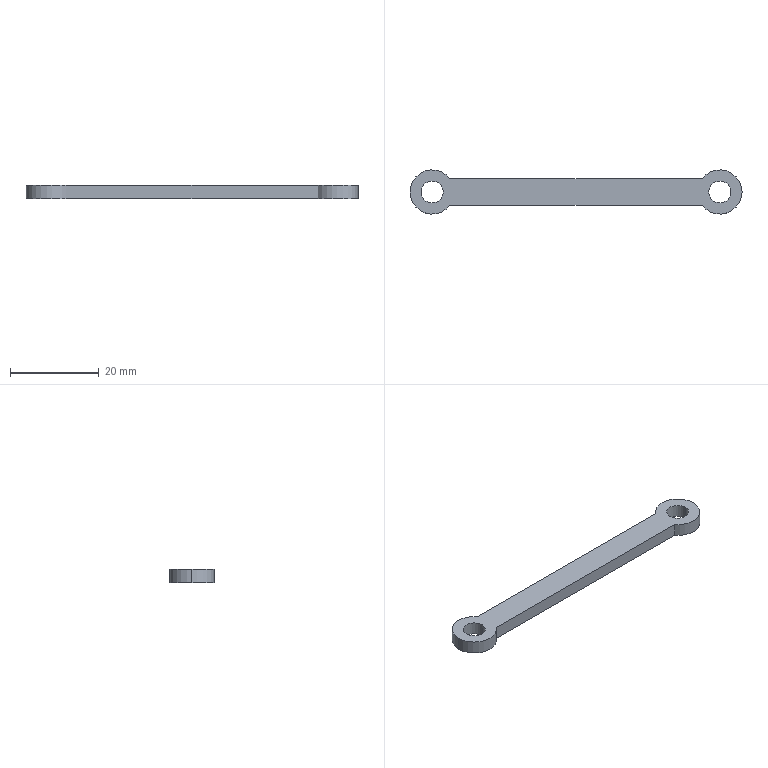Part | SolidWorks | features Extrusion 1 | 1 solid | 11 faces | box 75 x 10 x 3 mm | volume 1355 mm3 | cylinder 7 | plane 4 | commonest cylinder face diameters 5 x4 10 x3
STEP:
#1=CARTESIAN_POINT('',(62.5,0.,3.));
#2=VERTEX_POINT('',#1);
#3=CARTESIAN_POINT('',(67.5,0.,3.));
#4=VERTEX_POINT('',#3);
#5=CARTESIAN_POINT('',(65.,0.,3.));
#6=DIRECTION('',(0.,0.,1.));
#7=DIRECTION('',(1.,0.,0.));
#8=AXIS2_PLACEMENT_3D('',#5,#6,#7);
#9=CIRCLE('',#8,2.5);
#10=EDGE_CURVE('',#2,#4,#9,.T.);
#11=ORIENTED_EDGE('',*,*,#10,.T.);
#12=CARTESIAN_POINT('',(67.5,0.,0.));
#13=VERTEX_POINT('',#12);
#14=CARTESIAN_POINT('',(67.5,0.,3.));
#15=DIRECTION('',(0.,0.,-1.));
#16=VECTOR('',#15,1000.);
#17=LINE('',#14,#16);
#18=EDGE_CURVE('',#4,#13,#17,.T.);
#19=ORIENTED_EDGE('',*,*,#18,.T.);
#20=CARTESIAN_POINT('',(62.5,0.,0.));
#21=VERTEX_POINT('',#20);
#22=CARTESIAN_POINT('',(65.,0.,0.));
#23=DIRECTION('',(0.,0.,1.));
#24=DIRECTION('',(1.,0.,0.));
#25=AXIS2_PLACEMENT_3D('',#22,#23,#24);
#26=CIRCLE('',#25,2.5);
#27=EDGE_CURVE('',#21,#13,#26,.T.);
#28=ORIENTED_EDGE('',*,*,#27,.F.);
#29=CARTESIAN_POINT('',(62.5,0.,3.));
#30=DIRECTION('',(0.,0.,-1.));
#31=VECTOR('',#30,1000.);
#32=LINE('',#29,#31);
#33=EDGE_CURVE('',#2,#21,#32,.T.);
#34=ORIENTED_EDGE('',*,*,#33,.F.);
#35=EDGE_LOOP('',(#11,#19,#28,#34));
#36=FACE_OUTER_BOUND('',#35,.T.);
#37=CARTESIAN_POINT('',(65.,0.,3.));
#38=DIRECTION('',(0.,0.,-1.));
#39=DIRECTION('',(-1.,0.,0.));
#40=AXIS2_PLACEMENT_3D('',#37,#38,#39);
#41=CYLINDRICAL_SURFACE('',#40,2.5);
#42=ADVANCED_FACE('',(#36),#41,.F.);
#43=CARTESIAN_POINT('',(-2.5,0.,3.));
#44=VERTEX_POINT('',#43);
#45=CARTESIAN_POINT('',(2.5,0.,3.));
#46=VERTEX_POINT('',#45);
#47=CARTESIAN_POINT('',(0.,0.,3.));
#48=DIRECTION('',(0.,0.,1.));
#49=DIRECTION('',(1.,0.,0.));
#50=AXIS2_PLACEMENT_3D('',#47,#48,#49);
#51=CIRCLE('',#50,2.5);
#52=EDGE_CURVE('',#44,#46,#51,.T.);
#53=ORIENTED_EDGE('',*,*,#52,.T.);
#54=CARTESIAN_POINT('',(2.5,0.,0.));
#55=VERTEX_POINT('',#54);
#56=CARTESIAN_POINT('',(2.5,0.,3.));
#57=DIRECTION('',(0.,0.,-1.));
#58=VECTOR('',#57,1000.);
#59=LINE('',#56,#58);
#60=EDGE_CURVE('',#46,#55,#59,.T.);
#61=ORIENTED_EDGE('',*,*,#60,.T.);
#62=CARTESIAN_POINT('',(-2.5,0.,0.));
#63=VERTEX_POINT('',#62);
#64=CARTESIAN_POINT('',(0.,0.,0.));
#65=DIRECTION('',(0.,0.,1.));
#66=DIRECTION('',(1.,0.,0.));
#67=AXIS2_PLACEMENT_3D('',#64,#65,#66);
#68=CIRCLE('',#67,2.5);
#69=EDGE_CURVE('',#63,#55,#68,.T.);
#70=ORIENTED_EDGE('',*,*,#69,.F.);
#71=CARTESIAN_POINT('',(-2.5,0.,3.));
#72=DIRECTION('',(0.,0.,-1.));
#73=VECTOR('',#72,1000.);
#74=LINE('',#71,#73);
#75=EDGE_CURVE('',#44,#63,#74,.T.);
#76=ORIENTED_EDGE('',*,*,#75,.F.);
#77=EDGE_LOOP('',(#53,#61,#70,#76));
#78=FACE_OUTER_BOUND('',#77,.T.);
#79=CARTESIAN_POINT('',(0.,0.,3.));
#80=DIRECTION('',(0.,0.,-1.));
#81=DIRECTION('',(-1.,0.,0.));
#82=AXIS2_PLACEMENT_3D('',#79,#80,#81);
#83=CYLINDRICAL_SURFACE('',#82,2.5);
#84=ADVANCED_FACE('',(#78),#83,.F.);
#85=CARTESIAN_POINT('',(-5.,0.,3.));
#86=VERTEX_POINT('',#85);
#87=CARTESIAN_POINT('',(4.,-3.,3.));
#88=VERTEX_POINT('',#87);
#89=CARTESIAN_POINT('',(0.,0.,3.));
#90=DIRECTION('',(0.,0.,1.));
#91=DIRECTION('',(1.,0.,0.));
#92=AXIS2_PLACEMENT_3D('',#89,#90,#91);
#93=CIRCLE('',#92,5.);
#94=EDGE_CURVE('',#86,#88,#93,.T.);
#95=ORIENTED_EDGE('',*,*,#94,.F.);
#96=CARTESIAN_POINT('',(-5.,0.,0.));
#97=VERTEX_POINT('',#96);
#98=CARTESIAN_POINT('',(-5.,0.,3.));
#99=DIRECTION('',(0.,0.,-1.));
#100=VECTOR('',#99,1000.);
#101=LINE('',#98,#100);
#102=EDGE_CURVE('',#86,#97,#101,.T.);
#103=ORIENTED_EDGE('',*,*,#102,.T.);
#104=CARTESIAN_POINT('',(4.,-3.,0.));
#105=VERTEX_POINT('',#104);
#106=CARTESIAN_POINT('',(0.,0.,0.));
#107=DIRECTION('',(0.,0.,1.));
#108=DIRECTION('',(1.,0.,0.));
#109=AXIS2_PLACEMENT_3D('',#106,#107,#108);
#110=CIRCLE('',#109,5.);
#111=EDGE_CURVE('',#97,#105,#110,.T.);
#112=ORIENTED_EDGE('',*,*,#111,.T.);
#113=CARTESIAN_POINT('',(4.,-3.,3.));
#114=DIRECTION('',(0.,0.,-1.));
#115=VECTOR('',#114,1000.);
#116=LINE('',#113,#115);
#117=EDGE_CURVE('',#88,#105,#116,.T.);
#118=ORIENTED_EDGE('',*,*,#117,.F.);
#119=EDGE_LOOP('',(#95,#103,#112,#118));
#120=FACE_OUTER_BOUND('',#119,.T.);
#121=CARTESIAN_POINT('',(0.,0.,3.));
#122=DIRECTION('',(0.,0.,-1.));
#123=DIRECTION('',(-1.,0.,0.));
#124=AXIS2_PLACEMENT_3D('',#121,#122,#123);
#125=CYLINDRICAL_SURFACE('',#124,5.);
#126=ADVANCED_FACE('',(#120),#125,.T.);
#127=ORIENTED_EDGE('',*,*,#52,.F.);
#128=CARTESIAN_POINT('',(0.,0.,3.));
#129=DIRECTION('',(0.,0.,1.));
#130=DIRECTION('',(1.,0.,0.));
#131=AXIS2_PLACEMENT_3D('',#128,#129,#130);
#132=CIRCLE('',#131,2.5);
#133=EDGE_CURVE('',#46,#44,#132,.T.);
#134=ORIENTED_EDGE('',*,*,#133,.F.);
#135=EDGE_LOOP('',(#127,#134));
#136=FACE_BOUND('',#135,.T.);
#137=CARTESIAN_POINT('',(61.,-3.,3.));
#138=VERTEX_POINT('',#137);
#139=CARTESIAN_POINT('',(61.,3.,3.));
#140=VERTEX_POINT('',#139);
#141=CARTESIAN_POINT('',(65.,0.,3.));
#142=DIRECTION('',(0.,0.,1.));
#143=DIRECTION('',(1.,0.,0.));
#144=AXIS2_PLACEMENT_3D('',#141,#142,#143);
#145=CIRCLE('',#144,5.);
#146=EDGE_CURVE('',#138,#140,#145,.T.);
#147=ORIENTED_EDGE('',*,*,#146,.T.);
#148=CARTESIAN_POINT('',(4.,3.,3.));
#149=VERTEX_POINT('',#148);
#150=CARTESIAN_POINT('',(4.,3.,3.));
#151=DIRECTION('',(-1.,0.,0.));
#152=VECTOR('',#151,1000.);
#153=LINE('',#150,#152);
#154=EDGE_CURVE('',#140,#149,#153,.T.);
#155=ORIENTED_EDGE('',*,*,#154,.T.);
#156=CARTESIAN_POINT('',(0.,0.,3.));
#157=DIRECTION('',(0.,0.,1.));
#158=DIRECTION('',(1.,0.,0.));
#159=AXIS2_PLACEMENT_3D('',#156,#157,#158);
#160=CIRCLE('',#159,5.);
#161=EDGE_CURVE('',#149,#86,#160,.T.);
#162=ORIENTED_EDGE('',*,*,#161,.T.);
#163=ORIENTED_EDGE('',*,*,#94,.T.);
#164=CARTESIAN_POINT('',(4.,-3.,3.));
#165=DIRECTION('',(1.,0.,0.));
#166=VECTOR('',#165,1000.);
#167=LINE('',#164,#166);
#168=EDGE_CURVE('',#88,#138,#167,.T.);
#169=ORIENTED_EDGE('',*,*,#168,.T.);
#170=EDGE_LOOP('',(#147,#155,#162,#163,#169));
#171=FACE_OUTER_BOUND('',#170,.T.);
#172=ORIENTED_EDGE('',*,*,#10,.F.);
#173=CARTESIAN_POINT('',(65.,0.,3.));
#174=DIRECTION('',(0.,0.,1.));
#175=DIRECTION('',(1.,0.,0.));
#176=AXIS2_PLACEMENT_3D('',#173,#174,#175);
#177=CIRCLE('',#176,2.5);
#178=EDGE_CURVE('',#4,#2,#177,.T.);
#179=ORIENTED_EDGE('',*,*,#178,.F.);
#180=EDGE_LOOP('',(#172,#179));
#181=FACE_BOUND('',#180,.T.);
#182=CARTESIAN_POINT('',(65.,0.,3.));
#183=DIRECTION('',(0.,0.,1.));
#184=DIRECTION('',(1.,0.,0.));
#185=AXIS2_PLACEMENT_3D('',#182,#183,#184);
#186=PLANE('',#185);
#187=ADVANCED_FACE('',(#136,#171,#181),#186,.T.);
#188=CARTESIAN_POINT('',(61.,-3.,0.));
#189=VERTEX_POINT('',#188);
#190=CARTESIAN_POINT('',(61.,3.,0.));
#191=VERTEX_POINT('',#190);
#192=CARTESIAN_POINT('',(65.,0.,0.));
#193=DIRECTION('',(0.,0.,1.));
#194=DIRECTION('',(1.,0.,0.));
#195=AXIS2_PLACEMENT_3D('',#192,#193,#194);
#196=CIRCLE('',#195,5.);
#197=EDGE_CURVE('',#189,#191,#196,.T.);
#198=ORIENTED_EDGE('',*,*,#197,.F.);
#199=CARTESIAN_POINT('',(4.,-3.,0.));
#200=DIRECTION('',(1.,0.,0.));
#201=VECTOR('',#200,1000.);
#202=LINE('',#199,#201);
#203=EDGE_CURVE('',#105,#189,#202,.T.);
#204=ORIENTED_EDGE('',*,*,#203,.F.);
#205=ORIENTED_EDGE('',*,*,#111,.F.);
#206=CARTESIAN_POINT('',(4.,3.,0.));
#207=VERTEX_POINT('',#206);
#208=CARTESIAN_POINT('',(0.,0.,0.));
#209=DIRECTION('',(0.,0.,1.));
#210=DIRECTION('',(1.,0.,0.));
#211=AXIS2_PLACEMENT_3D('',#208,#209,#210);
#212=CIRCLE('',#211,5.);
#213=EDGE_CURVE('',#207,#97,#212,.T.);
#214=ORIENTED_EDGE('',*,*,#213,.F.);
#215=CARTESIAN_POINT('',(4.,3.,0.));
#216=DIRECTION('',(-1.,0.,0.));
#217=VECTOR('',#216,1000.);
#218=LINE('',#215,#217);
#219=EDGE_CURVE('',#191,#207,#218,.T.);
#220=ORIENTED_EDGE('',*,*,#219,.F.);
#221=EDGE_LOOP('',(#198,#204,#205,#214,#220));
#222=FACE_OUTER_BOUND('',#221,.T.);
#223=ORIENTED_EDGE('',*,*,#69,.T.);
#224=CARTESIAN_POINT('',(0.,0.,0.));
#225=DIRECTION('',(0.,0.,1.));
#226=DIRECTION('',(1.,0.,0.));
#227=AXIS2_PLACEMENT_3D('',#224,#225,#226);
#228=CIRCLE('',#227,2.5);
#229=EDGE_CURVE('',#55,#63,#228,.T.);
#230=ORIENTED_EDGE('',*,*,#229,.T.);
#231=EDGE_LOOP('',(#223,#230));
#232=FACE_BOUND('',#231,.T.);
#233=ORIENTED_EDGE('',*,*,#27,.T.);
#234=CARTESIAN_POINT('',(65.,0.,0.));
#235=DIRECTION('',(0.,0.,1.));
#236=DIRECTION('',(1.,0.,0.));
#237=AXIS2_PLACEMENT_3D('',#234,#235,#236);
#238=CIRCLE('',#237,2.5);
#239=EDGE_CURVE('',#13,#21,#238,.T.);
#240=ORIENTED_EDGE('',*,*,#239,.T.);
#241=EDGE_LOOP('',(#233,#240));
#242=FACE_BOUND('',#241,.T.);
#243=CARTESIAN_POINT('',(65.,0.,0.));
#244=DIRECTION('',(0.,0.,1.));
#245=DIRECTION('',(1.,0.,0.));
#246=AXIS2_PLACEMENT_3D('',#243,#244,#245);
#247=PLANE('',#246);
#248=ADVANCED_FACE('',(#222,#232,#242),#247,.F.);
#249=ORIENTED_EDGE('',*,*,#197,.T.);
#250=CARTESIAN_POINT('',(61.,3.,3.));
#251=DIRECTION('',(0.,0.,-1.));
#252=VECTOR('',#251,1000.);
#253=LINE('',#250,#252);
#254=EDGE_CURVE('',#140,#191,#253,.T.);
#255=ORIENTED_EDGE('',*,*,#254,.F.);
#256=ORIENTED_EDGE('',*,*,#146,.F.);
#257=CARTESIAN_POINT('',(61.,-3.,3.));
#258=DIRECTION('',(0.,0.,-1.));
#259=VECTOR('',#258,1000.);
#260=LINE('',#257,#259);
#261=EDGE_CURVE('',#138,#189,#260,.T.);
#262=ORIENTED_EDGE('',*,*,#261,.T.);
#263=EDGE_LOOP('',(#249,#255,#256,#262));
#264=FACE_OUTER_BOUND('',#263,.T.);
#265=CARTESIAN_POINT('',(65.,0.,3.));
#266=DIRECTION('',(0.,0.,-1.));
#267=DIRECTION('',(-1.,0.,0.));
#268=AXIS2_PLACEMENT_3D('',#265,#266,#267);
#269=CYLINDRICAL_SURFACE('',#268,5.);
#270=ADVANCED_FACE('',(#264),#269,.T.);
#271=ORIENTED_EDGE('',*,*,#219,.T.);
#272=CARTESIAN_POINT('',(4.,3.,3.));
#273=DIRECTION('',(0.,0.,-1.));
#274=VECTOR('',#273,1000.);
#275=LINE('',#272,#274);
#276=EDGE_CURVE('',#149,#207,#275,.T.);
#277=ORIENTED_EDGE('',*,*,#276,.F.);
#278=ORIENTED_EDGE('',*,*,#154,.F.);
#279=ORIENTED_EDGE('',*,*,#254,.T.);
#280=EDGE_LOOP('',(#271,#277,#278,#279));
#281=FACE_OUTER_BOUND('',#280,.T.);
#282=CARTESIAN_POINT('',(4.,3.,3.));
#283=DIRECTION('',(0.,-1.,0.));
#284=DIRECTION('',(0.,0.,-1.));
#285=AXIS2_PLACEMENT_3D('',#282,#283,#284);
#286=PLANE('',#285);
#287=ADVANCED_FACE('',(#281),#286,.F.);
#288=ORIENTED_EDGE('',*,*,#102,.F.);
#289=ORIENTED_EDGE('',*,*,#161,.F.);
#290=ORIENTED_EDGE('',*,*,#276,.T.);
#291=ORIENTED_EDGE('',*,*,#213,.T.);
#292=EDGE_LOOP('',(#288,#289,#290,#291));
#293=FACE_OUTER_BOUND('',#292,.T.);
#294=CARTESIAN_POINT('',(0.,0.,3.));
#295=DIRECTION('',(0.,0.,-1.));
#296=DIRECTION('',(-1.,0.,0.));
#297=AXIS2_PLACEMENT_3D('',#294,#295,#296);
#298=CYLINDRICAL_SURFACE('',#297,5.);
#299=ADVANCED_FACE('',(#293),#298,.T.);
#300=ORIENTED_EDGE('',*,*,#203,.T.);
#301=ORIENTED_EDGE('',*,*,#261,.F.);
#302=ORIENTED_EDGE('',*,*,#168,.F.);
#303=ORIENTED_EDGE('',*,*,#117,.T.);
#304=EDGE_LOOP('',(#300,#301,#302,#303));
#305=FACE_OUTER_BOUND('',#304,.T.);
#306=CARTESIAN_POINT('',(4.,-3.,3.));
#307=DIRECTION('',(0.,1.,0.));
#308=DIRECTION('',(0.,0.,1.));
#309=AXIS2_PLACEMENT_3D('',#306,#307,#308);
#310=PLANE('',#309);
#311=ADVANCED_FACE('',(#305),#310,.F.);
#312=ORIENTED_EDGE('',*,*,#60,.F.);
#313=ORIENTED_EDGE('',*,*,#133,.T.);
#314=ORIENTED_EDGE('',*,*,#75,.T.);
#315=ORIENTED_EDGE('',*,*,#229,.F.);
#316=EDGE_LOOP('',(#312,#313,#314,#315));
#317=FACE_OUTER_BOUND('',#316,.T.);
#318=CARTESIAN_POINT('',(0.,0.,3.));
#319=DIRECTION('',(0.,0.,-1.));
#320=DIRECTION('',(-1.,0.,0.));
#321=AXIS2_PLACEMENT_3D('',#318,#319,#320);
#322=CYLINDRICAL_SURFACE('',#321,2.5);
#323=ADVANCED_FACE('',(#317),#322,.F.);
#324=ORIENTED_EDGE('',*,*,#18,.F.);
#325=ORIENTED_EDGE('',*,*,#178,.T.);
#326=ORIENTED_EDGE('',*,*,#33,.T.);
#327=ORIENTED_EDGE('',*,*,#239,.F.);
#328=EDGE_LOOP('',(#324,#325,#326,#327));
#329=FACE_OUTER_BOUND('',#328,.T.);
#330=CARTESIAN_POINT('',(65.,0.,3.));
#331=DIRECTION('',(0.,0.,-1.));
#332=DIRECTION('',(-1.,0.,0.));
#333=AXIS2_PLACEMENT_3D('',#330,#331,#332);
#334=CYLINDRICAL_SURFACE('',#333,2.5);
#335=ADVANCED_FACE('',(#329),#334,.F.);
#336=CLOSED_SHELL('',(#42,#84,#126,#187,#248,#270,#287,#299,#311,#323,#335));
#337=MANIFOLD_SOLID_BREP('',#336);
#338=CARTESIAN_POINT('',(0.,0.,0.));
#339=DIRECTION('',(0.,0.,1.));
#340=DIRECTION('',(1.,0.,0.));
#341=AXIS2_PLACEMENT_3D('',#338,#339,#340);
#342=(LENGTH_UNIT()NAMED_UNIT(*)SI_UNIT(.MILLI.,.METRE.));
#343=UNCERTAINTY_MEASURE_WITH_UNIT(LENGTH_MEASURE(0.00001),#342,'','');
#344=(NAMED_UNIT(*)PLANE_ANGLE_UNIT()SI_UNIT($,.RADIAN.));
#345=(NAMED_UNIT(*)SI_UNIT($,.STERADIAN.)SOLID_ANGLE_UNIT());
#346=(GEOMETRIC_REPRESENTATION_CONTEXT(3)GLOBAL_UNCERTAINTY_ASSIGNED_CONTEXT((#343))GLOBAL_UNIT_ASSIGNED_CONTEXT((#342,#344,#345))REPRESENTATION_CONTEXT('',''));
#347=ADVANCED_BREP_SHAPE_REPRESENTATION('',(#337,#341),#346);